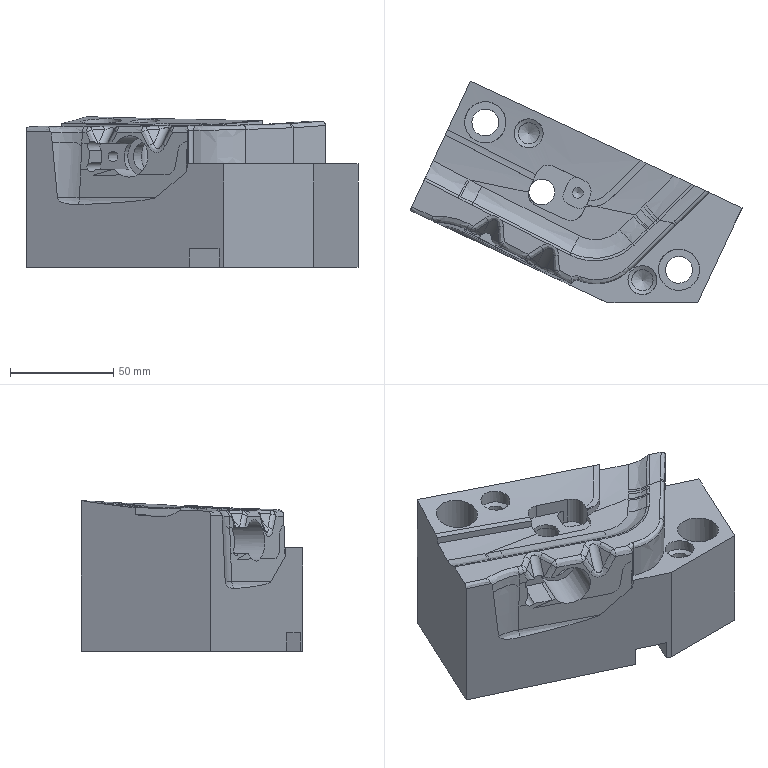Part | STEP file | gslz 2016.10.28-13_id1450_x_t | 1 solid | 145 faces | box 160.575 x 107.178 x 72.851 mm | volume 541622 mm3 | spline 67 | plane 35 | cylinder 30 | cone 6 | sphere 4 | other 3 | commonest cylinder face diameters 12.4 x4 8 x3 14 x3 20 x3 5 x2 5.2 x2